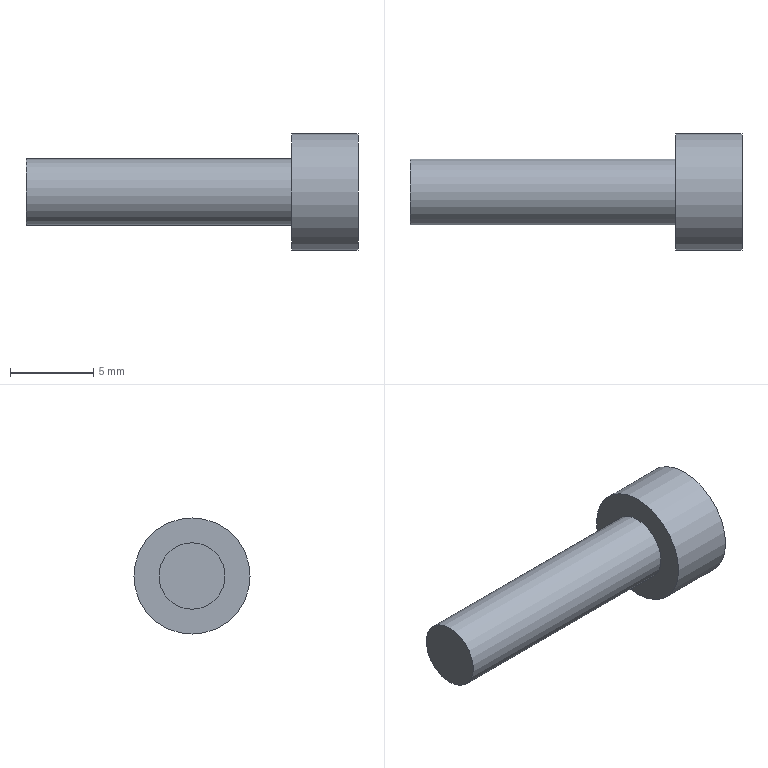Part | NX | features Bolt-1_5003_015_HTLA24S5M150-E-10 2 | 1 solid | 18 faces | box 20 x 7 x 7 mm | volume 337.371 mm3 | plane 15 | cylinder 2 | cone 1 | commonest cylinder face diameters 4 x1 7 x1
STEP:
#1=CARTESIAN_POINT('',(228.025,133.526,-156.));
#2=VERTEX_POINT('',#1);
#3=CARTESIAN_POINT('',(228.025,133.526,-152.5));
#4=DIRECTION('',(1.,0.,0.));
#5=DIRECTION('',(0.,0.,-1.));
#6=AXIS2_PLACEMENT_3D('',#3,#4,#5);
#7=CIRCLE('',#6,3.5);
#8=EDGE_CURVE('',#2,#2,#7,.T.);
#9=ORIENTED_EDGE('',*,*,#8,.T.);
#10=EDGE_LOOP('',(#9));
#11=FACE_BOUND('',#10,.T.);
#12=CARTESIAN_POINT('',(228.025,131.794,-152.5));
#13=VERTEX_POINT('',#12);
#14=CARTESIAN_POINT('',(228.025,132.66,-154.));
#15=VERTEX_POINT('',#14);
#16=CARTESIAN_POINT('',(228.025,131.794,-152.5));
#17=DIRECTION('',(0.,0.5,-0.866));
#18=VECTOR('',#17,1000.);
#19=LINE('',#16,#18);
#20=EDGE_CURVE('',#13,#15,#19,.T.);
#21=ORIENTED_EDGE('',*,*,#20,.F.);
#22=CARTESIAN_POINT('',(228.025,132.66,-151.));
#23=VERTEX_POINT('',#22);
#24=CARTESIAN_POINT('',(228.025,132.66,-151.));
#25=DIRECTION('',(0.,-0.5,-0.866));
#26=VECTOR('',#25,1000.);
#27=LINE('',#24,#26);
#28=EDGE_CURVE('',#23,#13,#27,.T.);
#29=ORIENTED_EDGE('',*,*,#28,.F.);
#30=CARTESIAN_POINT('',(228.025,134.392,-151.));
#31=VERTEX_POINT('',#30);
#32=CARTESIAN_POINT('',(228.025,134.392,-151.));
#33=DIRECTION('',(0.,-1.,0.));
#34=VECTOR('',#33,1000.);
#35=LINE('',#32,#34);
#36=EDGE_CURVE('',#31,#23,#35,.T.);
#37=ORIENTED_EDGE('',*,*,#36,.F.);
#38=CARTESIAN_POINT('',(228.025,135.258,-152.5));
#39=VERTEX_POINT('',#38);
#40=CARTESIAN_POINT('',(228.025,135.258,-152.5));
#41=DIRECTION('',(0.,-0.5,0.866));
#42=VECTOR('',#41,1000.);
#43=LINE('',#40,#42);
#44=EDGE_CURVE('',#39,#31,#43,.T.);
#45=ORIENTED_EDGE('',*,*,#44,.F.);
#46=CARTESIAN_POINT('',(228.025,134.392,-154.));
#47=VERTEX_POINT('',#46);
#48=CARTESIAN_POINT('',(228.025,134.392,-154.));
#49=DIRECTION('',(0.,0.5,0.866));
#50=VECTOR('',#49,1000.);
#51=LINE('',#48,#50);
#52=EDGE_CURVE('',#47,#39,#51,.T.);
#53=ORIENTED_EDGE('',*,*,#52,.F.);
#54=CARTESIAN_POINT('',(228.025,132.66,-154.));
#55=DIRECTION('',(0.,1.,0.));
#56=VECTOR('',#55,1000.);
#57=LINE('',#54,#56);
#58=EDGE_CURVE('',#15,#47,#57,.T.);
#59=ORIENTED_EDGE('',*,*,#58,.F.);
#60=EDGE_LOOP('',(#21,#29,#37,#45,#53,#59));
#61=FACE_BOUND('',#60,.T.);
#62=CARTESIAN_POINT('',(228.025,133.526,-152.5));
#63=DIRECTION('',(-1.,0.,0.));
#64=DIRECTION('',(0.,0.,1.));
#65=AXIS2_PLACEMENT_3D('',#62,#63,#64);
#66=PLANE('',#65);
#67=ADVANCED_FACE('',(#11,#61),#66,.F.);
#68=ORIENTED_EDGE('',*,*,#8,.F.);
#69=EDGE_LOOP('',(#68));
#70=FACE_BOUND('',#69,.T.);
#71=CARTESIAN_POINT('',(224.025,133.526,-156.));
#72=VERTEX_POINT('',#71);
#73=CARTESIAN_POINT('',(224.025,133.526,-152.5));
#74=DIRECTION('',(1.,0.,0.));
#75=DIRECTION('',(0.,0.,-1.));
#76=AXIS2_PLACEMENT_3D('',#73,#74,#75);
#77=CIRCLE('',#76,3.5);
#78=EDGE_CURVE('',#72,#72,#77,.T.);
#79=ORIENTED_EDGE('',*,*,#78,.T.);
#80=EDGE_LOOP('',(#79));
#81=FACE_BOUND('',#80,.T.);
#82=CARTESIAN_POINT('',(228.025,133.526,-152.5));
#83=DIRECTION('',(1.,0.,0.));
#84=DIRECTION('',(0.,0.,-1.));
#85=AXIS2_PLACEMENT_3D('',#82,#83,#84);
#86=CYLINDRICAL_SURFACE('',#85,3.5);
#87=ADVANCED_FACE('',(#70,#81),#86,.T.);
#88=ORIENTED_EDGE('',*,*,#78,.F.);
#89=EDGE_LOOP('',(#88));
#90=FACE_BOUND('',#89,.T.);
#91=CARTESIAN_POINT('',(224.025,133.526,-154.5));
#92=VERTEX_POINT('',#91);
#93=CARTESIAN_POINT('',(224.025,133.526,-152.5));
#94=DIRECTION('',(1.,0.,0.));
#95=DIRECTION('',(0.,0.,-1.));
#96=AXIS2_PLACEMENT_3D('',#93,#94,#95);
#97=CIRCLE('',#96,2.);
#98=EDGE_CURVE('',#92,#92,#97,.T.);
#99=ORIENTED_EDGE('',*,*,#98,.T.);
#100=EDGE_LOOP('',(#99));
#101=FACE_BOUND('',#100,.T.);
#102=CARTESIAN_POINT('',(224.025,133.526,-149.));
#103=DIRECTION('',(1.,0.,0.));
#104=DIRECTION('',(0.,0.,-1.));
#105=AXIS2_PLACEMENT_3D('',#102,#103,#104);
#106=PLANE('',#105);
#107=ADVANCED_FACE('',(#90,#101),#106,.F.);
#108=ORIENTED_EDGE('',*,*,#98,.F.);
#109=EDGE_LOOP('',(#108));
#110=FACE_BOUND('',#109,.T.);
#111=CARTESIAN_POINT('',(208.025,133.526,-154.5));
#112=VERTEX_POINT('',#111);
#113=CARTESIAN_POINT('',(208.025,133.526,-152.5));
#114=DIRECTION('',(1.,0.,0.));
#115=DIRECTION('',(0.,0.,-1.));
#116=AXIS2_PLACEMENT_3D('',#113,#114,#115);
#117=CIRCLE('',#116,2.);
#118=EDGE_CURVE('',#112,#112,#117,.T.);
#119=ORIENTED_EDGE('',*,*,#118,.T.);
#120=EDGE_LOOP('',(#119));
#121=FACE_BOUND('',#120,.T.);
#122=CARTESIAN_POINT('',(228.025,133.526,-152.5));
#123=DIRECTION('',(1.,0.,0.));
#124=DIRECTION('',(0.,0.,-1.));
#125=AXIS2_PLACEMENT_3D('',#122,#123,#124);
#126=CYLINDRICAL_SURFACE('',#125,2.);
#127=ADVANCED_FACE('',(#110,#121),#126,.T.);
#128=ORIENTED_EDGE('',*,*,#118,.F.);
#129=EDGE_LOOP('',(#128));
#130=FACE_BOUND('',#129,.T.);
#131=CARTESIAN_POINT('',(208.025,133.526,-150.5));
#132=DIRECTION('',(1.,0.,0.));
#133=DIRECTION('',(0.,0.,-1.));
#134=AXIS2_PLACEMENT_3D('',#131,#132,#133);
#135=PLANE('',#134);
#136=ADVANCED_FACE('',(#130),#135,.F.);
#137=CARTESIAN_POINT('',(226.025,132.66,-151.));
#138=VERTEX_POINT('',#137);
#139=CARTESIAN_POINT('',(226.025,132.227,-151.75));
#140=VERTEX_POINT('',#139);
#141=CARTESIAN_POINT('',(226.025,132.66,-151.));
#142=DIRECTION('',(0.,-0.5,-0.866));
#143=VECTOR('',#142,1000.);
#144=LINE('',#141,#143);
#145=EDGE_CURVE('',#138,#140,#144,.T.);
#146=ORIENTED_EDGE('',*,*,#145,.F.);
#147=CARTESIAN_POINT('',(226.025,132.66,-151.));
#148=DIRECTION('',(1.,0.,0.));
#149=VECTOR('',#148,1000.);
#150=LINE('',#147,#149);
#151=EDGE_CURVE('',#138,#23,#150,.T.);
#152=ORIENTED_EDGE('',*,*,#151,.T.);
#153=ORIENTED_EDGE('',*,*,#28,.T.);
#154=CARTESIAN_POINT('',(226.025,131.794,-152.5));
#155=VERTEX_POINT('',#154);
#156=CARTESIAN_POINT('',(226.025,131.794,-152.5));
#157=DIRECTION('',(1.,0.,0.));
#158=VECTOR('',#157,1000.);
#159=LINE('',#156,#158);
#160=EDGE_CURVE('',#155,#13,#159,.T.);
#161=ORIENTED_EDGE('',*,*,#160,.F.);
#162=CARTESIAN_POINT('',(226.025,132.66,-151.));
#163=DIRECTION('',(0.,-0.5,-0.866));
#164=VECTOR('',#163,1000.);
#165=LINE('',#162,#164);
#166=EDGE_CURVE('',#140,#155,#165,.T.);
#167=ORIENTED_EDGE('',*,*,#166,.F.);
#168=EDGE_LOOP('',(#146,#152,#153,#161,#167));
#169=FACE_BOUND('',#168,.T.);
#170=CARTESIAN_POINT('',(226.025,132.66,-151.));
#171=DIRECTION('',(0.,-0.866,0.5));
#172=DIRECTION('',(0.,-0.5,-0.866));
#173=AXIS2_PLACEMENT_3D('',#170,#171,#172);
#174=PLANE('',#173);
#175=ADVANCED_FACE('',(#169),#174,.F.);
#176=CARTESIAN_POINT('',(226.025,134.392,-151.));
#177=VERTEX_POINT('',#176);
#178=CARTESIAN_POINT('',(226.025,133.526,-151.));
#179=VERTEX_POINT('',#178);
#180=CARTESIAN_POINT('',(226.025,134.392,-151.));
#181=DIRECTION('',(0.,-1.,0.));
#182=VECTOR('',#181,1000.);
#183=LINE('',#180,#182);
#184=EDGE_CURVE('',#177,#179,#183,.T.);
#185=ORIENTED_EDGE('',*,*,#184,.F.);
#186=CARTESIAN_POINT('',(226.025,134.392,-151.));
#187=DIRECTION('',(1.,0.,0.));
#188=VECTOR('',#187,1000.);
#189=LINE('',#186,#188);
#190=EDGE_CURVE('',#177,#31,#189,.T.);
#191=ORIENTED_EDGE('',*,*,#190,.T.);
#192=ORIENTED_EDGE('',*,*,#36,.T.);
#193=ORIENTED_EDGE('',*,*,#151,.F.);
#194=CARTESIAN_POINT('',(226.025,134.392,-151.));
#195=DIRECTION('',(0.,-1.,0.));
#196=VECTOR('',#195,1000.);
#197=LINE('',#194,#196);
#198=EDGE_CURVE('',#179,#138,#197,.T.);
#199=ORIENTED_EDGE('',*,*,#198,.F.);
#200=EDGE_LOOP('',(#185,#191,#192,#193,#199));
#201=FACE_BOUND('',#200,.T.);
#202=CARTESIAN_POINT('',(226.025,134.392,-151.));
#203=DIRECTION('',(0.,0.,1.));
#204=DIRECTION('',(0.,-1.,0.));
#205=AXIS2_PLACEMENT_3D('',#202,#203,#204);
#206=PLANE('',#205);
#207=ADVANCED_FACE('',(#201),#206,.F.);
#208=CARTESIAN_POINT('',(226.025,135.258,-152.5));
#209=VERTEX_POINT('',#208);
#210=CARTESIAN_POINT('',(226.025,134.825,-151.75));
#211=VERTEX_POINT('',#210);
#212=CARTESIAN_POINT('',(226.025,135.258,-152.5));
#213=DIRECTION('',(0.,-0.5,0.866));
#214=VECTOR('',#213,1000.);
#215=LINE('',#212,#214);
#216=EDGE_CURVE('',#209,#211,#215,.T.);
#217=ORIENTED_EDGE('',*,*,#216,.F.);
#218=CARTESIAN_POINT('',(226.025,135.258,-152.5));
#219=DIRECTION('',(1.,0.,0.));
#220=VECTOR('',#219,1000.);
#221=LINE('',#218,#220);
#222=EDGE_CURVE('',#209,#39,#221,.T.);
#223=ORIENTED_EDGE('',*,*,#222,.T.);
#224=ORIENTED_EDGE('',*,*,#44,.T.);
#225=ORIENTED_EDGE('',*,*,#190,.F.);
#226=CARTESIAN_POINT('',(226.025,135.258,-152.5));
#227=DIRECTION('',(0.,-0.5,0.866));
#228=VECTOR('',#227,1000.);
#229=LINE('',#226,#228);
#230=EDGE_CURVE('',#211,#177,#229,.T.);
#231=ORIENTED_EDGE('',*,*,#230,.F.);
#232=EDGE_LOOP('',(#217,#223,#224,#225,#231));
#233=FACE_BOUND('',#232,.T.);
#234=CARTESIAN_POINT('',(226.025,135.258,-152.5));
#235=DIRECTION('',(0.,0.866,0.5));
#236=DIRECTION('',(0.,-0.5,0.866));
#237=AXIS2_PLACEMENT_3D('',#234,#235,#236);
#238=PLANE('',#237);
#239=ADVANCED_FACE('',(#233),#238,.F.);
#240=CARTESIAN_POINT('',(226.025,134.392,-154.));
#241=VERTEX_POINT('',#240);
#242=CARTESIAN_POINT('',(226.025,134.825,-153.25));
#243=VERTEX_POINT('',#242);
#244=CARTESIAN_POINT('',(226.025,134.392,-154.));
#245=DIRECTION('',(0.,0.5,0.866));
#246=VECTOR('',#245,1000.);
#247=LINE('',#244,#246);
#248=EDGE_CURVE('',#241,#243,#247,.T.);
#249=ORIENTED_EDGE('',*,*,#248,.F.);
#250=CARTESIAN_POINT('',(226.025,134.392,-154.));
#251=DIRECTION('',(1.,0.,0.));
#252=VECTOR('',#251,1000.);
#253=LINE('',#250,#252);
#254=EDGE_CURVE('',#241,#47,#253,.T.);
#255=ORIENTED_EDGE('',*,*,#254,.T.);
#256=ORIENTED_EDGE('',*,*,#52,.T.);
#257=ORIENTED_EDGE('',*,*,#222,.F.);
#258=CARTESIAN_POINT('',(226.025,134.392,-154.));
#259=DIRECTION('',(0.,0.5,0.866));
#260=VECTOR('',#259,1000.);
#261=LINE('',#258,#260);
#262=EDGE_CURVE('',#243,#209,#261,.T.);
#263=ORIENTED_EDGE('',*,*,#262,.F.);
#264=EDGE_LOOP('',(#249,#255,#256,#257,#263));
#265=FACE_BOUND('',#264,.T.);
#266=CARTESIAN_POINT('',(226.025,134.392,-154.));
#267=DIRECTION('',(0.,0.866,-0.5));
#268=DIRECTION('',(0.,0.5,0.866));
#269=AXIS2_PLACEMENT_3D('',#266,#267,#268);
#270=PLANE('',#269);
#271=ADVANCED_FACE('',(#265),#270,.F.);
#272=CARTESIAN_POINT('',(226.025,132.66,-154.));
#273=VERTEX_POINT('',#272);
#274=CARTESIAN_POINT('',(226.025,133.526,-154.));
#275=VERTEX_POINT('',#274);
#276=CARTESIAN_POINT('',(226.025,132.66,-154.));
#277=DIRECTION('',(0.,1.,0.));
#278=VECTOR('',#277,1000.);
#279=LINE('',#276,#278);
#280=EDGE_CURVE('',#273,#275,#279,.T.);
#281=ORIENTED_EDGE('',*,*,#280,.F.);
#282=CARTESIAN_POINT('',(226.025,132.66,-154.));
#283=DIRECTION('',(1.,0.,0.));
#284=VECTOR('',#283,1000.);
#285=LINE('',#282,#284);
#286=EDGE_CURVE('',#273,#15,#285,.T.);
#287=ORIENTED_EDGE('',*,*,#286,.T.);
#288=ORIENTED_EDGE('',*,*,#58,.T.);
#289=ORIENTED_EDGE('',*,*,#254,.F.);
#290=CARTESIAN_POINT('',(226.025,132.66,-154.));
#291=DIRECTION('',(0.,1.,0.));
#292=VECTOR('',#291,1000.);
#293=LINE('',#290,#292);
#294=EDGE_CURVE('',#275,#241,#293,.T.);
#295=ORIENTED_EDGE('',*,*,#294,.F.);
#296=EDGE_LOOP('',(#281,#287,#288,#289,#295));
#297=FACE_BOUND('',#296,.T.);
#298=CARTESIAN_POINT('',(226.025,132.66,-154.));
#299=DIRECTION('',(0.,0.,-1.));
#300=DIRECTION('',(0.,1.,0.));
#301=AXIS2_PLACEMENT_3D('',#298,#299,#300);
#302=PLANE('',#301);
#303=ADVANCED_FACE('',(#297),#302,.F.);
#304=CARTESIAN_POINT('',(226.025,132.227,-153.25));
#305=VERTEX_POINT('',#304);
#306=CARTESIAN_POINT('',(226.025,131.794,-152.5));
#307=DIRECTION('',(0.,0.5,-0.866));
#308=VECTOR('',#307,1000.);
#309=LINE('',#306,#308);
#310=EDGE_CURVE('',#155,#305,#309,.T.);
#311=ORIENTED_EDGE('',*,*,#310,.F.);
#312=ORIENTED_EDGE('',*,*,#160,.T.);
#313=ORIENTED_EDGE('',*,*,#20,.T.);
#314=ORIENTED_EDGE('',*,*,#286,.F.);
#315=CARTESIAN_POINT('',(226.025,131.794,-152.5));
#316=DIRECTION('',(0.,0.5,-0.866));
#317=VECTOR('',#316,1000.);
#318=LINE('',#315,#317);
#319=EDGE_CURVE('',#305,#273,#318,.T.);
#320=ORIENTED_EDGE('',*,*,#319,.F.);
#321=EDGE_LOOP('',(#311,#312,#313,#314,#320));
#322=FACE_BOUND('',#321,.T.);
#323=CARTESIAN_POINT('',(226.025,131.794,-152.5));
#324=DIRECTION('',(0.,-0.866,-0.5));
#325=DIRECTION('',(0.,0.5,-0.866));
#326=AXIS2_PLACEMENT_3D('',#323,#324,#325);
#327=PLANE('',#326);
#328=ADVANCED_FACE('',(#322),#327,.F.);
#329=ORIENTED_EDGE('',*,*,#230,.T.);
#330=ORIENTED_EDGE('',*,*,#184,.T.);
#331=CARTESIAN_POINT('',(226.025,133.526,-152.5));
#332=DIRECTION('',(1.,0.,0.));
#333=DIRECTION('',(0.,0.,-1.));
#334=AXIS2_PLACEMENT_3D('',#331,#332,#333);
#335=CIRCLE('',#334,1.5);
#336=EDGE_CURVE('',#211,#179,#335,.T.);
#337=ORIENTED_EDGE('',*,*,#336,.F.);
#338=EDGE_LOOP('',(#329,#330,#337));
#339=FACE_BOUND('',#338,.T.);
#340=CARTESIAN_POINT('',(226.025,133.526,-152.5));
#341=DIRECTION('',(1.,0.,0.));
#342=DIRECTION('',(0.,1.,0.));
#343=AXIS2_PLACEMENT_3D('',#340,#341,#342);
#344=PLANE('',#343);
#345=ADVANCED_FACE('',(#339),#344,.T.);
#346=ORIENTED_EDGE('',*,*,#198,.T.);
#347=ORIENTED_EDGE('',*,*,#145,.T.);
#348=CARTESIAN_POINT('',(226.025,133.526,-152.5));
#349=DIRECTION('',(1.,0.,0.));
#350=DIRECTION('',(0.,0.,-1.));
#351=AXIS2_PLACEMENT_3D('',#348,#349,#350);
#352=CIRCLE('',#351,1.5);
#353=EDGE_CURVE('',#179,#140,#352,.T.);
#354=ORIENTED_EDGE('',*,*,#353,.F.);
#355=EDGE_LOOP('',(#346,#347,#354));
#356=FACE_BOUND('',#355,.T.);
#357=CARTESIAN_POINT('',(226.025,133.526,-152.5));
#358=DIRECTION('',(1.,0.,0.));
#359=DIRECTION('',(0.,1.,0.));
#360=AXIS2_PLACEMENT_3D('',#357,#358,#359);
#361=PLANE('',#360);
#362=ADVANCED_FACE('',(#356),#361,.T.);
#363=ORIENTED_EDGE('',*,*,#166,.T.);
#364=ORIENTED_EDGE('',*,*,#310,.T.);
#365=CARTESIAN_POINT('',(226.025,133.526,-152.5));
#366=DIRECTION('',(1.,0.,0.));
#367=DIRECTION('',(0.,0.,-1.));
#368=AXIS2_PLACEMENT_3D('',#365,#366,#367);
#369=CIRCLE('',#368,1.5);
#370=EDGE_CURVE('',#140,#305,#369,.T.);
#371=ORIENTED_EDGE('',*,*,#370,.F.);
#372=EDGE_LOOP('',(#363,#364,#371));
#373=FACE_BOUND('',#372,.T.);
#374=CARTESIAN_POINT('',(226.025,133.526,-152.5));
#375=DIRECTION('',(1.,0.,0.));
#376=DIRECTION('',(0.,1.,0.));
#377=AXIS2_PLACEMENT_3D('',#374,#375,#376);
#378=PLANE('',#377);
#379=ADVANCED_FACE('',(#373),#378,.T.);
#380=ORIENTED_EDGE('',*,*,#319,.T.);
#381=ORIENTED_EDGE('',*,*,#280,.T.);
#382=CARTESIAN_POINT('',(226.025,133.526,-152.5));
#383=DIRECTION('',(1.,0.,0.));
#384=DIRECTION('',(0.,0.,-1.));
#385=AXIS2_PLACEMENT_3D('',#382,#383,#384);
#386=CIRCLE('',#385,1.5);
#387=EDGE_CURVE('',#305,#275,#386,.T.);
#388=ORIENTED_EDGE('',*,*,#387,.F.);
#389=EDGE_LOOP('',(#380,#381,#388));
#390=FACE_BOUND('',#389,.T.);
#391=CARTESIAN_POINT('',(226.025,133.526,-152.5));
#392=DIRECTION('',(1.,0.,0.));
#393=DIRECTION('',(0.,1.,0.));
#394=AXIS2_PLACEMENT_3D('',#391,#392,#393);
#395=PLANE('',#394);
#396=ADVANCED_FACE('',(#390),#395,.T.);
#397=ORIENTED_EDGE('',*,*,#294,.T.);
#398=ORIENTED_EDGE('',*,*,#248,.T.);
#399=CARTESIAN_POINT('',(226.025,133.526,-152.5));
#400=DIRECTION('',(1.,0.,0.));
#401=DIRECTION('',(0.,0.,-1.));
#402=AXIS2_PLACEMENT_3D('',#399,#400,#401);
#403=CIRCLE('',#402,1.5);
#404=EDGE_CURVE('',#275,#243,#403,.T.);
#405=ORIENTED_EDGE('',*,*,#404,.F.);
#406=EDGE_LOOP('',(#397,#398,#405));
#407=FACE_BOUND('',#406,.T.);
#408=CARTESIAN_POINT('',(226.025,133.526,-152.5));
#409=DIRECTION('',(1.,0.,0.));
#410=DIRECTION('',(0.,1.,0.));
#411=AXIS2_PLACEMENT_3D('',#408,#409,#410);
#412=PLANE('',#411);
#413=ADVANCED_FACE('',(#407),#412,.T.);
#414=ORIENTED_EDGE('',*,*,#262,.T.);
#415=ORIENTED_EDGE('',*,*,#216,.T.);
#416=CARTESIAN_POINT('',(226.025,133.526,-152.5));
#417=DIRECTION('',(1.,0.,0.));
#418=DIRECTION('',(0.,0.,-1.));
#419=AXIS2_PLACEMENT_3D('',#416,#417,#418);
#420=CIRCLE('',#419,1.5);
#421=EDGE_CURVE('',#243,#211,#420,.T.);
#422=ORIENTED_EDGE('',*,*,#421,.F.);
#423=EDGE_LOOP('',(#414,#415,#422));
#424=FACE_BOUND('',#423,.T.);
#425=CARTESIAN_POINT('',(226.025,133.526,-152.5));
#426=DIRECTION('',(1.,0.,0.));
#427=DIRECTION('',(0.,1.,0.));
#428=AXIS2_PLACEMENT_3D('',#425,#426,#427);
#429=PLANE('',#428);
#430=ADVANCED_FACE('',(#424),#429,.T.);
#431=ORIENTED_EDGE('',*,*,#404,.T.);
#432=ORIENTED_EDGE('',*,*,#421,.T.);
#433=ORIENTED_EDGE('',*,*,#336,.T.);
#434=ORIENTED_EDGE('',*,*,#353,.T.);
#435=ORIENTED_EDGE('',*,*,#370,.T.);
#436=ORIENTED_EDGE('',*,*,#387,.T.);
#437=EDGE_LOOP('',(#431,#432,#433,#434,#435,#436));
#438=FACE_BOUND('',#437,.T.);
#439=CARTESIAN_POINT('',(225.159,133.526,-152.5));
#440=VERTEX_POINT('',#439);
#441=VERTEX_LOOP('',#440);
#442=FACE_BOUND('',#441,.T.);
#443=CARTESIAN_POINT('',(225.159,133.526,-152.5));
#444=DIRECTION('',(1.,0.,0.));
#445=DIRECTION('',(0.,0.,-1.));
#446=AXIS2_PLACEMENT_3D('',#443,#444,#445);
#447=CONICAL_SURFACE('',#446,0.,1.047);
#448=ADVANCED_FACE('',(#438,#442),#447,.F.);
#449=CLOSED_SHELL('',(#67,#87,#107,#127,#136,#175,#207,#239,#271,#303,#328,#345,#362,#379,#396,#413,#430,#448));
#450=MANIFOLD_SOLID_BREP('',#449);
#451=(LENGTH_UNIT()NAMED_UNIT(*)SI_UNIT(.MILLI.,.METRE.));
#452=UNCERTAINTY_MEASURE_WITH_UNIT(LENGTH_MEASURE(0.00001),#451,'','');
#453=(NAMED_UNIT(*)PLANE_ANGLE_UNIT()SI_UNIT($,.RADIAN.));
#454=(NAMED_UNIT(*)SI_UNIT($,.STERADIAN.)SOLID_ANGLE_UNIT());
#455=(GEOMETRIC_REPRESENTATION_CONTEXT(3)GLOBAL_UNCERTAINTY_ASSIGNED_CONTEXT((#452))GLOBAL_UNIT_ASSIGNED_CONTEXT((#451,#453,#454))REPRESENTATION_CONTEXT('',''));
#456=ADVANCED_BREP_SHAPE_REPRESENTATION('',(#450),#455);